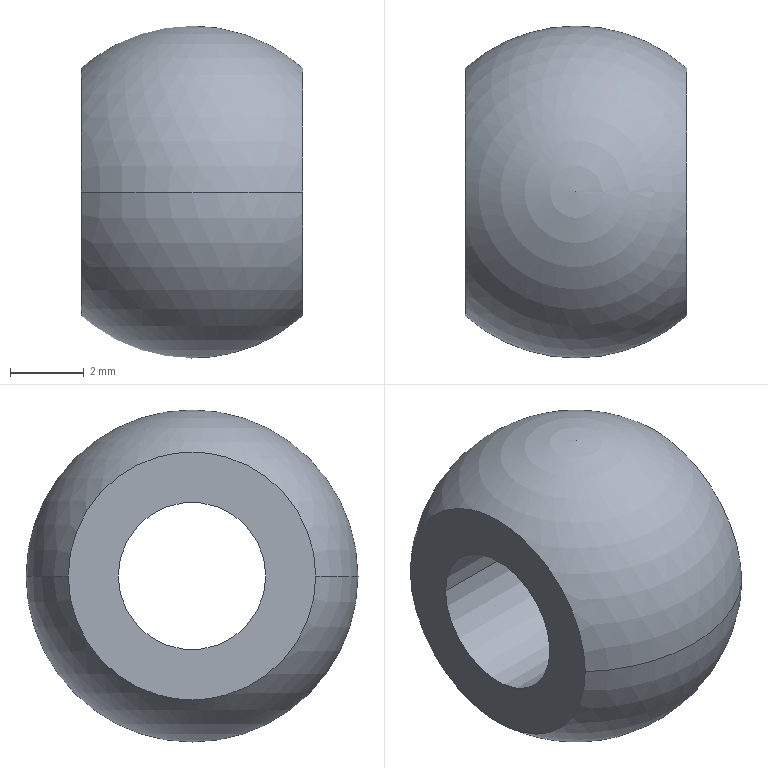Part | SolidWorks | features ICE 2, Revolution 1 | 1 solid | 6 faces | box 6 x 9 x 9 mm | volume 249.757 mm3 | cylinder 2 | sphere 2 | plane 2 | commonest cylinder face diameters 4 x2
STEP:
#1=CARTESIAN_POINT('',(3.,2.,0.));
#2=VERTEX_POINT('',#1);
#3=CARTESIAN_POINT('',(3.,-2.,0.));
#4=VERTEX_POINT('',#3);
#5=CARTESIAN_POINT('',(3.,0.,0.));
#6=DIRECTION('',(-1.,0.,0.));
#7=DIRECTION('',(0.,-1.,0.));
#8=AXIS2_PLACEMENT_3D('',#5,#6,#7);
#9=CIRCLE('',#8,2.);
#10=EDGE_CURVE('',#2,#4,#9,.T.);
#11=ORIENTED_EDGE('',*,*,#10,.F.);
#12=CARTESIAN_POINT('',(-3.,2.,0.));
#13=VERTEX_POINT('',#12);
#14=CARTESIAN_POINT('',(17.,2.,0.));
#15=DIRECTION('',(-1.,0.,0.));
#16=VECTOR('',#15,1000.);
#17=LINE('',#14,#16);
#18=EDGE_CURVE('',#2,#13,#17,.T.);
#19=ORIENTED_EDGE('',*,*,#18,.T.);
#20=CARTESIAN_POINT('',(-3.,-2.,0.));
#21=VERTEX_POINT('',#20);
#22=CARTESIAN_POINT('',(-3.,0.,0.));
#23=DIRECTION('',(-1.,0.,0.));
#24=DIRECTION('',(0.,-1.,0.));
#25=AXIS2_PLACEMENT_3D('',#22,#23,#24);
#26=CIRCLE('',#25,2.);
#27=EDGE_CURVE('',#13,#21,#26,.T.);
#28=ORIENTED_EDGE('',*,*,#27,.T.);
#29=CARTESIAN_POINT('',(17.,-2.,0.));
#30=DIRECTION('',(-1.,0.,0.));
#31=VECTOR('',#30,1000.);
#32=LINE('',#29,#31);
#33=EDGE_CURVE('',#4,#21,#32,.T.);
#34=ORIENTED_EDGE('',*,*,#33,.F.);
#35=EDGE_LOOP('',(#11,#19,#28,#34));
#36=FACE_OUTER_BOUND('',#35,.T.);
#37=CARTESIAN_POINT('',(17.,0.,0.));
#38=DIRECTION('',(-1.,0.,0.));
#39=DIRECTION('',(0.,-1.,0.));
#40=AXIS2_PLACEMENT_3D('',#37,#38,#39);
#41=CYLINDRICAL_SURFACE('',#40,2.);
#42=ADVANCED_FACE('',(#36),#41,.F.);
#43=CARTESIAN_POINT('',(0.,-4.5,0.));
#44=VERTEX_POINT('',#43);
#45=CARTESIAN_POINT('',(3.,-3.354,0.));
#46=VERTEX_POINT('',#45);
#47=CARTESIAN_POINT('',(0.,0.,0.));
#48=DIRECTION('',(0.,0.,1.));
#49=DIRECTION('',(1.,0.,0.));
#50=AXIS2_PLACEMENT_3D('',#47,#48,#49);
#51=CIRCLE('',#50,4.5);
#52=EDGE_CURVE('',#44,#46,#51,.T.);
#53=ORIENTED_EDGE('',*,*,#52,.F.);
#54=CARTESIAN_POINT('',(-3.,-3.354,0.));
#55=VERTEX_POINT('',#54);
#56=CARTESIAN_POINT('',(0.,0.,0.));
#57=DIRECTION('',(0.,0.,-1.));
#58=DIRECTION('',(-1.,0.,0.));
#59=AXIS2_PLACEMENT_3D('',#56,#57,#58);
#60=CIRCLE('',#59,4.5);
#61=EDGE_CURVE('',#44,#55,#60,.T.);
#62=ORIENTED_EDGE('',*,*,#61,.T.);
#63=CARTESIAN_POINT('',(-3.,3.354,0.));
#64=VERTEX_POINT('',#63);
#65=CARTESIAN_POINT('',(-3.,0.,0.));
#66=DIRECTION('',(1.,0.,0.));
#67=DIRECTION('',(0.,1.,0.));
#68=AXIS2_PLACEMENT_3D('',#65,#66,#67);
#69=CIRCLE('',#68,3.354);
#70=EDGE_CURVE('',#55,#64,#69,.T.);
#71=ORIENTED_EDGE('',*,*,#70,.T.);
#72=CARTESIAN_POINT('',(0.,4.5,0.));
#73=VERTEX_POINT('',#72);
#74=CARTESIAN_POINT('',(0.,0.,0.));
#75=DIRECTION('',(0.,0.,-1.));
#76=DIRECTION('',(-1.,0.,0.));
#77=AXIS2_PLACEMENT_3D('',#74,#75,#76);
#78=CIRCLE('',#77,4.5);
#79=EDGE_CURVE('',#64,#73,#78,.T.);
#80=ORIENTED_EDGE('',*,*,#79,.T.);
#81=CARTESIAN_POINT('',(3.,3.354,0.));
#82=VERTEX_POINT('',#81);
#83=CARTESIAN_POINT('',(0.,0.,0.));
#84=DIRECTION('',(0.,0.,1.));
#85=DIRECTION('',(1.,0.,0.));
#86=AXIS2_PLACEMENT_3D('',#83,#84,#85);
#87=CIRCLE('',#86,4.5);
#88=EDGE_CURVE('',#82,#73,#87,.T.);
#89=ORIENTED_EDGE('',*,*,#88,.F.);
#90=CARTESIAN_POINT('',(3.,0.,0.));
#91=DIRECTION('',(-1.,0.,0.));
#92=DIRECTION('',(0.,-1.,0.));
#93=AXIS2_PLACEMENT_3D('',#90,#91,#92);
#94=CIRCLE('',#93,3.354);
#95=EDGE_CURVE('',#82,#46,#94,.T.);
#96=ORIENTED_EDGE('',*,*,#95,.T.);
#97=EDGE_LOOP('',(#53,#62,#71,#80,#89,#96));
#98=FACE_OUTER_BOUND('',#97,.T.);
#99=CARTESIAN_POINT('',(0.,0.,0.));
#100=DIRECTION('',(0.,0.,-1.));
#101=DIRECTION('',(1.,0.,0.));
#102=AXIS2_PLACEMENT_3D('',#99,#100,#101);
#103=SPHERICAL_SURFACE('',#102,4.5);
#104=ADVANCED_FACE('',(#98),#103,.T.);
#105=ORIENTED_EDGE('',*,*,#61,.F.);
#106=ORIENTED_EDGE('',*,*,#52,.T.);
#107=CARTESIAN_POINT('',(3.,0.,0.));
#108=DIRECTION('',(-1.,0.,0.));
#109=DIRECTION('',(0.,-1.,0.));
#110=AXIS2_PLACEMENT_3D('',#107,#108,#109);
#111=CIRCLE('',#110,3.354);
#112=EDGE_CURVE('',#46,#82,#111,.T.);
#113=ORIENTED_EDGE('',*,*,#112,.T.);
#114=ORIENTED_EDGE('',*,*,#88,.T.);
#115=ORIENTED_EDGE('',*,*,#79,.F.);
#116=CARTESIAN_POINT('',(-3.,0.,0.));
#117=DIRECTION('',(1.,0.,0.));
#118=DIRECTION('',(0.,1.,0.));
#119=AXIS2_PLACEMENT_3D('',#116,#117,#118);
#120=CIRCLE('',#119,3.354);
#121=EDGE_CURVE('',#64,#55,#120,.T.);
#122=ORIENTED_EDGE('',*,*,#121,.T.);
#123=EDGE_LOOP('',(#105,#106,#113,#114,#115,#122));
#124=FACE_OUTER_BOUND('',#123,.T.);
#125=CARTESIAN_POINT('',(0.,0.,0.));
#126=DIRECTION('',(0.,0.,-1.));
#127=DIRECTION('',(1.,0.,0.));
#128=AXIS2_PLACEMENT_3D('',#125,#126,#127);
#129=SPHERICAL_SURFACE('',#128,4.5);
#130=ADVANCED_FACE('',(#124),#129,.T.);
#131=CARTESIAN_POINT('',(3.,0.,0.));
#132=DIRECTION('',(-1.,0.,0.));
#133=DIRECTION('',(0.,-1.,0.));
#134=AXIS2_PLACEMENT_3D('',#131,#132,#133);
#135=CIRCLE('',#134,2.);
#136=EDGE_CURVE('',#4,#2,#135,.T.);
#137=ORIENTED_EDGE('',*,*,#136,.T.);
#138=ORIENTED_EDGE('',*,*,#10,.T.);
#139=EDGE_LOOP('',(#137,#138));
#140=FACE_BOUND('',#139,.T.);
#141=ORIENTED_EDGE('',*,*,#112,.F.);
#142=ORIENTED_EDGE('',*,*,#95,.F.);
#143=EDGE_LOOP('',(#141,#142));
#144=FACE_OUTER_BOUND('',#143,.T.);
#145=CARTESIAN_POINT('',(3.,4.618,-10.));
#146=DIRECTION('',(-1.,0.,0.));
#147=DIRECTION('',(0.,-1.,0.));
#148=AXIS2_PLACEMENT_3D('',#145,#146,#147);
#149=PLANE('',#148);
#150=ADVANCED_FACE('',(#140,#144),#149,.F.);
#151=CARTESIAN_POINT('',(-3.,0.,0.));
#152=DIRECTION('',(-1.,0.,0.));
#153=DIRECTION('',(0.,-1.,0.));
#154=AXIS2_PLACEMENT_3D('',#151,#152,#153);
#155=CIRCLE('',#154,2.);
#156=EDGE_CURVE('',#21,#13,#155,.T.);
#157=ORIENTED_EDGE('',*,*,#156,.F.);
#158=ORIENTED_EDGE('',*,*,#27,.F.);
#159=EDGE_LOOP('',(#157,#158));
#160=FACE_BOUND('',#159,.T.);
#161=ORIENTED_EDGE('',*,*,#121,.F.);
#162=ORIENTED_EDGE('',*,*,#70,.F.);
#163=EDGE_LOOP('',(#161,#162));
#164=FACE_OUTER_BOUND('',#163,.T.);
#165=CARTESIAN_POINT('',(-3.,4.618,-10.));
#166=DIRECTION('',(1.,0.,0.));
#167=DIRECTION('',(0.,1.,0.));
#168=AXIS2_PLACEMENT_3D('',#165,#166,#167);
#169=PLANE('',#168);
#170=ADVANCED_FACE('',(#160,#164),#169,.F.);
#171=ORIENTED_EDGE('',*,*,#18,.F.);
#172=ORIENTED_EDGE('',*,*,#136,.F.);
#173=ORIENTED_EDGE('',*,*,#33,.T.);
#174=ORIENTED_EDGE('',*,*,#156,.T.);
#175=EDGE_LOOP('',(#171,#172,#173,#174));
#176=FACE_OUTER_BOUND('',#175,.T.);
#177=CARTESIAN_POINT('',(17.,0.,0.));
#178=DIRECTION('',(-1.,0.,0.));
#179=DIRECTION('',(0.,-1.,0.));
#180=AXIS2_PLACEMENT_3D('',#177,#178,#179);
#181=CYLINDRICAL_SURFACE('',#180,2.);
#182=ADVANCED_FACE('',(#176),#181,.F.);
#183=CLOSED_SHELL('',(#42,#104,#130,#150,#170,#182));
#184=MANIFOLD_SOLID_BREP('',#183);
#185=CARTESIAN_POINT('',(0.,0.,0.));
#186=DIRECTION('',(0.,0.,1.));
#187=DIRECTION('',(1.,0.,0.));
#188=AXIS2_PLACEMENT_3D('',#185,#186,#187);
#189=(LENGTH_UNIT()NAMED_UNIT(*)SI_UNIT(.MILLI.,.METRE.));
#190=UNCERTAINTY_MEASURE_WITH_UNIT(LENGTH_MEASURE(0.00001),#189,'','');
#191=(NAMED_UNIT(*)PLANE_ANGLE_UNIT()SI_UNIT($,.RADIAN.));
#192=(NAMED_UNIT(*)SI_UNIT($,.STERADIAN.)SOLID_ANGLE_UNIT());
#193=(GEOMETRIC_REPRESENTATION_CONTEXT(3)GLOBAL_UNCERTAINTY_ASSIGNED_CONTEXT((#190))GLOBAL_UNIT_ASSIGNED_CONTEXT((#189,#191,#192))REPRESENTATION_CONTEXT('',''));
#194=ADVANCED_BREP_SHAPE_REPRESENTATION('',(#184,#188),#193);